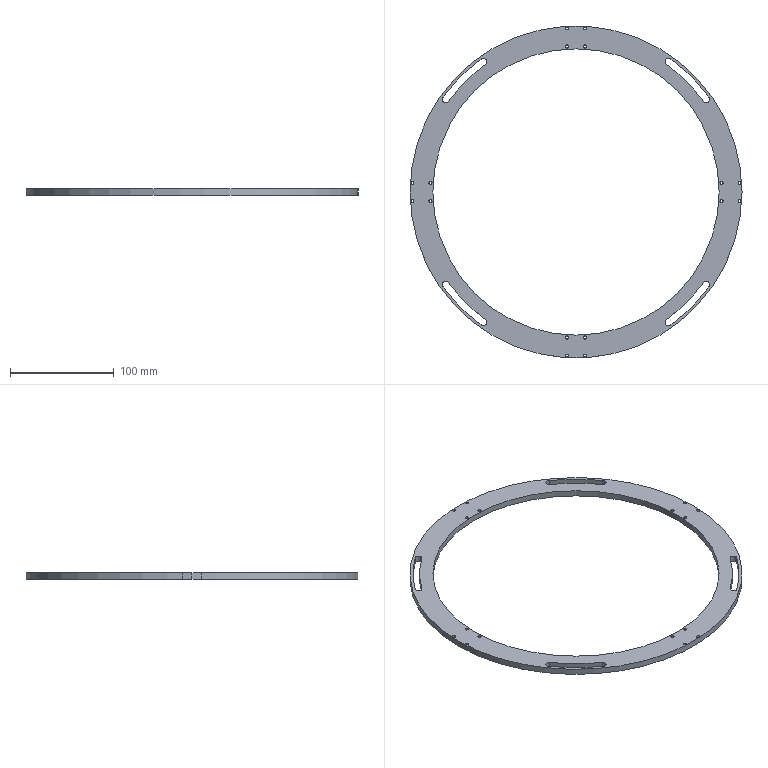Part | SolidWorks | features Extrusion 1 | 1 solid | 58 faces | box 319.492 x 319.492 x 6 mm | volume 113822 mm3 | cylinder 56 | plane 2 | commonest cylinder face diameters 3 x32 6.598 x12 301 x4 314 x4 275.492 x2 319.492 x2